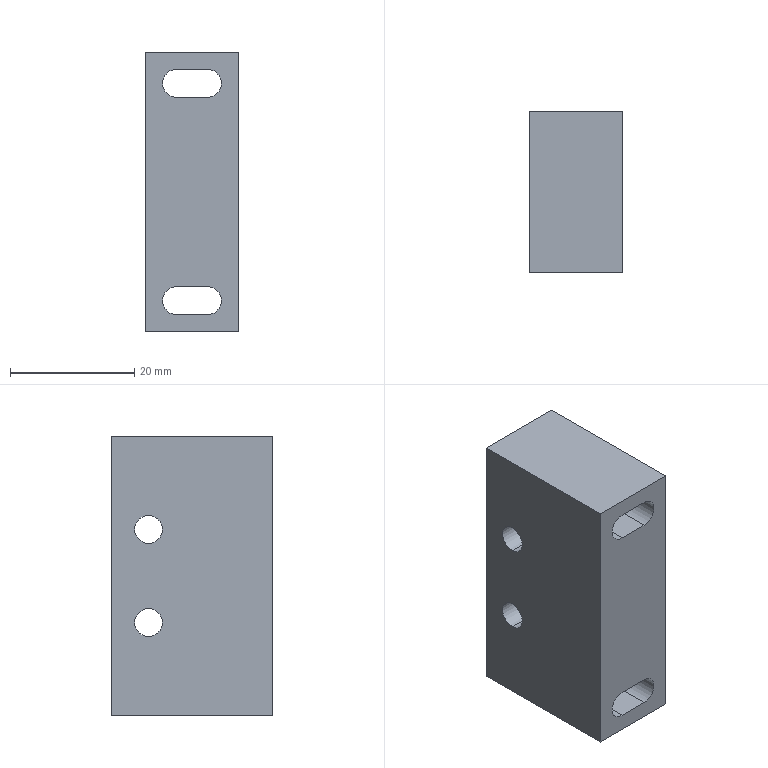Part | STEP file | 0246_221_Block | 1 solid | 18 faces | box 15 x 26 x 45 mm | volume 15076 mm3 | plane 10 | cylinder 8 | commonest cylinder face diameters 4.5 x8
STEP:
#1=CARTESIAN_POINT('',(0.,0.,0.));
#2=DIRECTION('',(0.,0.,1.));
#3=DIRECTION('',(1.,0.,0.));
#4=AXIS2_PLACEMENT_3D('',#1,#2,#3);
#5=CARTESIAN_POINT('',(-15.,20.,5.25));
#6=VERTEX_POINT('',#5);
#7=CARTESIAN_POINT('',(0.,20.,5.25));
#8=VERTEX_POINT('',#7);
#9=CARTESIAN_POINT('',(0.,20.,5.25));
#10=DIRECTION('',(1.,0.,0.));
#11=VECTOR('',#10,1.);
#12=LINE('',#9,#11);
#13=CARTESIAN_POINT('',(0.,20.,7.5));
#14=DIRECTION('',(1.,0.,0.));
#15=DIRECTION('',(0.,0.,-1.));
#16=AXIS2_PLACEMENT_3D('',#13,#14,#15);
#17=CYLINDRICAL_SURFACE('',#16,2.25);
#18=CARTESIAN_POINT('',(6.283,0.));
#19=DIRECTION('',(0.,1.));
#20=VECTOR('',#19,1.);
#21=LINE('',#18,#20);
#22=(GEOMETRIC_REPRESENTATION_CONTEXT(2)PARAMETRIC_REPRESENTATION_CONTEXT()REPRESENTATION_CONTEXT('',''));
#23=DEFINITIONAL_REPRESENTATION('',(#21),#22);
#24=PCURVE('',#17,#23);
#25=CARTESIAN_POINT('',(0.,20.,7.5));
#26=DIRECTION('',(1.,0.,0.));
#27=DIRECTION('',(0.,0.,-1.));
#28=AXIS2_PLACEMENT_3D('',#25,#26,#27);
#29=CYLINDRICAL_SURFACE('',#28,2.25);
#30=CARTESIAN_POINT('',(0.,0.));
#31=DIRECTION('',(0.,1.));
#32=VECTOR('',#31,1.);
#33=LINE('',#30,#32);
#34=(GEOMETRIC_REPRESENTATION_CONTEXT(2)PARAMETRIC_REPRESENTATION_CONTEXT()REPRESENTATION_CONTEXT('',''));
#35=DEFINITIONAL_REPRESENTATION('',(#33),#34);
#36=PCURVE('',#29,#35);
#37=SURFACE_CURVE('',#12,(#24,#36),.PCURVE_S1.);
#38=EDGE_CURVE('',#6,#8,#37,.T.);
#39=ORIENTED_EDGE('',*,*,#38,.T.);
#40=CARTESIAN_POINT('',(0.,20.,9.75));
#41=VERTEX_POINT('',#40);
#42=CARTESIAN_POINT('',(0.,20.,7.5));
#43=DIRECTION('',(1.,0.,0.));
#44=DIRECTION('',(0.,0.,-1.));
#45=AXIS2_PLACEMENT_3D('',#42,#43,#44);
#46=CIRCLE('',#45,2.25);
#47=CARTESIAN_POINT('',(0.,0.));
#48=DIRECTION('',(1.,0.));
#49=VECTOR('',#48,1.);
#50=LINE('',#47,#49);
#51=(GEOMETRIC_REPRESENTATION_CONTEXT(2)PARAMETRIC_REPRESENTATION_CONTEXT()REPRESENTATION_CONTEXT('',''));
#52=DEFINITIONAL_REPRESENTATION('',(#50),#51);
#53=PCURVE('',#17,#52);
#54=CARTESIAN_POINT('',(0.,26.,-22.5));
#55=DIRECTION('',(-1.,0.,0.));
#56=DIRECTION('',(0.,0.,1.));
#57=AXIS2_PLACEMENT_3D('',#54,#55,#56);
#58=PLANE('',#57);
#59=CARTESIAN_POINT('',(27.75,-6.));
#60=CARTESIAN_POINT('',(27.75,-2.103));
#61=CARTESIAN_POINT('',(31.125,-4.051));
#62=CARTESIAN_POINT('',(34.5,-6.));
#63=CARTESIAN_POINT('',(31.125,-7.949));
#64=CARTESIAN_POINT('',(27.75,-9.897));
#65=CARTESIAN_POINT('',(27.75,-6.));
#66=(BOUNDED_CURVE()B_SPLINE_CURVE(2,(#59,#60,#61,#62,#63,#64,#65),.UNSPECIFIED.,.T.,.F.)B_SPLINE_CURVE_WITH_KNOTS((1,2,2,2,2,1),(-2.094,0.,2.094,4.189,6.283,8.378),.UNSPECIFIED.)CURVE()GEOMETRIC_REPRESENTATION_ITEM()RATIONAL_B_SPLINE_CURVE((1.,0.5,1.,0.5,1.,0.5,1.))REPRESENTATION_ITEM(''));
#67=(GEOMETRIC_REPRESENTATION_CONTEXT(2)PARAMETRIC_REPRESENTATION_CONTEXT()REPRESENTATION_CONTEXT('',''));
#68=DEFINITIONAL_REPRESENTATION('',(#66),#67);
#69=PCURVE('',#58,#68);
#70=SURFACE_CURVE('',#46,(#53,#69),.PCURVE_S1.);
#71=EDGE_CURVE('',#41,#8,#70,.T.);
#72=ORIENTED_EDGE('',*,*,#71,.F.);
#73=CARTESIAN_POINT('',(-15.,20.,9.75));
#74=VERTEX_POINT('',#73);
#75=CARTESIAN_POINT('',(0.,20.,9.75));
#76=DIRECTION('',(1.,0.,0.));
#77=VECTOR('',#76,1.);
#78=LINE('',#75,#77);
#79=CARTESIAN_POINT('',(3.142,0.));
#80=DIRECTION('',(0.,1.));
#81=VECTOR('',#80,1.);
#82=LINE('',#79,#81);
#83=(GEOMETRIC_REPRESENTATION_CONTEXT(2)PARAMETRIC_REPRESENTATION_CONTEXT()REPRESENTATION_CONTEXT('',''));
#84=DEFINITIONAL_REPRESENTATION('',(#82),#83);
#85=PCURVE('',#17,#84);
#86=CARTESIAN_POINT('',(3.142,0.));
#87=DIRECTION('',(0.,1.));
#88=VECTOR('',#87,1.);
#89=LINE('',#86,#88);
#90=(GEOMETRIC_REPRESENTATION_CONTEXT(2)PARAMETRIC_REPRESENTATION_CONTEXT()REPRESENTATION_CONTEXT('',''));
#91=DEFINITIONAL_REPRESENTATION('',(#89),#90);
#92=PCURVE('',#29,#91);
#93=SURFACE_CURVE('',#78,(#85,#92),.PCURVE_S1.);
#94=EDGE_CURVE('',#74,#41,#93,.T.);
#95=ORIENTED_EDGE('',*,*,#94,.F.);
#96=CARTESIAN_POINT('',(-15.,20.,7.5));
#97=DIRECTION('',(1.,0.,0.));
#98=DIRECTION('',(0.,0.,-1.));
#99=AXIS2_PLACEMENT_3D('',#96,#97,#98);
#100=CIRCLE('',#99,2.25);
#101=CARTESIAN_POINT('',(0.,-15.));
#102=DIRECTION('',(1.,0.));
#103=VECTOR('',#102,1.);
#104=LINE('',#101,#103);
#105=(GEOMETRIC_REPRESENTATION_CONTEXT(2)PARAMETRIC_REPRESENTATION_CONTEXT()REPRESENTATION_CONTEXT('',''));
#106=DEFINITIONAL_REPRESENTATION('',(#104),#105);
#107=PCURVE('',#17,#106);
#108=CARTESIAN_POINT('',(-15.,26.,-22.5));
#109=DIRECTION('',(1.,0.,0.));
#110=DIRECTION('',(0.,0.,-1.));
#111=AXIS2_PLACEMENT_3D('',#108,#109,#110);
#112=PLANE('',#111);
#113=CARTESIAN_POINT('',(-30.,-6.));
#114=DIRECTION('',(1.,0.));
#115=AXIS2_PLACEMENT_2D('',#113,#114);
#116=CIRCLE('',#115,2.25);
#117=(GEOMETRIC_REPRESENTATION_CONTEXT(2)PARAMETRIC_REPRESENTATION_CONTEXT()REPRESENTATION_CONTEXT('',''));
#118=DEFINITIONAL_REPRESENTATION('',(#116),#117);
#119=PCURVE('',#112,#118);
#120=SURFACE_CURVE('',#100,(#107,#119),.PCURVE_S1.);
#121=EDGE_CURVE('',#74,#6,#120,.T.);
#122=ORIENTED_EDGE('',*,*,#121,.T.);
#123=EDGE_LOOP('',(#39,#72,#95,#122));
#124=FACE_BOUND('',#123,.F.);
#125=ADVANCED_FACE('',(#124),#17,.F.);
#126=CARTESIAN_POINT('',(-15.,20.,-9.75));
#127=VERTEX_POINT('',#126);
#128=CARTESIAN_POINT('',(0.,20.,-9.75));
#129=VERTEX_POINT('',#128);
#130=CARTESIAN_POINT('',(0.,20.,-9.75));
#131=DIRECTION('',(1.,0.,0.));
#132=VECTOR('',#131,1.);
#133=LINE('',#130,#132);
#134=CARTESIAN_POINT('',(0.,20.,-7.5));
#135=DIRECTION('',(1.,0.,0.));
#136=DIRECTION('',(0.,0.,-1.));
#137=AXIS2_PLACEMENT_3D('',#134,#135,#136);
#138=CYLINDRICAL_SURFACE('',#137,2.25);
#139=CARTESIAN_POINT('',(6.283,0.));
#140=DIRECTION('',(0.,1.));
#141=VECTOR('',#140,1.);
#142=LINE('',#139,#141);
#143=(GEOMETRIC_REPRESENTATION_CONTEXT(2)PARAMETRIC_REPRESENTATION_CONTEXT()REPRESENTATION_CONTEXT('',''));
#144=DEFINITIONAL_REPRESENTATION('',(#142),#143);
#145=PCURVE('',#138,#144);
#146=CARTESIAN_POINT('',(0.,20.,-7.5));
#147=DIRECTION('',(1.,0.,0.));
#148=DIRECTION('',(0.,0.,-1.));
#149=AXIS2_PLACEMENT_3D('',#146,#147,#148);
#150=CYLINDRICAL_SURFACE('',#149,2.25);
#151=CARTESIAN_POINT('',(0.,0.));
#152=DIRECTION('',(0.,1.));
#153=VECTOR('',#152,1.);
#154=LINE('',#151,#153);
#155=(GEOMETRIC_REPRESENTATION_CONTEXT(2)PARAMETRIC_REPRESENTATION_CONTEXT()REPRESENTATION_CONTEXT('',''));
#156=DEFINITIONAL_REPRESENTATION('',(#154),#155);
#157=PCURVE('',#150,#156);
#158=SURFACE_CURVE('',#133,(#145,#157),.PCURVE_S1.);
#159=EDGE_CURVE('',#127,#129,#158,.T.);
#160=ORIENTED_EDGE('',*,*,#159,.T.);
#161=CARTESIAN_POINT('',(0.,20.,-5.25));
#162=VERTEX_POINT('',#161);
#163=CARTESIAN_POINT('',(0.,20.,-7.5));
#164=DIRECTION('',(1.,0.,0.));
#165=DIRECTION('',(0.,0.,-1.));
#166=AXIS2_PLACEMENT_3D('',#163,#164,#165);
#167=CIRCLE('',#166,2.25);
#168=CARTESIAN_POINT('',(0.,0.));
#169=DIRECTION('',(1.,0.));
#170=VECTOR('',#169,1.);
#171=LINE('',#168,#170);
#172=(GEOMETRIC_REPRESENTATION_CONTEXT(2)PARAMETRIC_REPRESENTATION_CONTEXT()REPRESENTATION_CONTEXT('',''));
#173=DEFINITIONAL_REPRESENTATION('',(#171),#172);
#174=PCURVE('',#138,#173);
#175=CARTESIAN_POINT('',(12.75,-6.));
#176=CARTESIAN_POINT('',(12.75,-2.103));
#177=CARTESIAN_POINT('',(16.125,-4.051));
#178=CARTESIAN_POINT('',(19.5,-6.));
#179=CARTESIAN_POINT('',(16.125,-7.949));
#180=CARTESIAN_POINT('',(12.75,-9.897));
#181=CARTESIAN_POINT('',(12.75,-6.));
#182=(BOUNDED_CURVE()B_SPLINE_CURVE(2,(#175,#176,#177,#178,#179,#180,#181),.UNSPECIFIED.,.T.,.F.)B_SPLINE_CURVE_WITH_KNOTS((1,2,2,2,2,1),(-2.094,0.,2.094,4.189,6.283,8.378),.UNSPECIFIED.)CURVE()GEOMETRIC_REPRESENTATION_ITEM()RATIONAL_B_SPLINE_CURVE((1.,0.5,1.,0.5,1.,0.5,1.))REPRESENTATION_ITEM(''));
#183=(GEOMETRIC_REPRESENTATION_CONTEXT(2)PARAMETRIC_REPRESENTATION_CONTEXT()REPRESENTATION_CONTEXT('',''));
#184=DEFINITIONAL_REPRESENTATION('',(#182),#183);
#185=PCURVE('',#58,#184);
#186=SURFACE_CURVE('',#167,(#174,#185),.PCURVE_S1.);
#187=EDGE_CURVE('',#162,#129,#186,.T.);
#188=ORIENTED_EDGE('',*,*,#187,.F.);
#189=CARTESIAN_POINT('',(-15.,20.,-5.25));
#190=VERTEX_POINT('',#189);
#191=CARTESIAN_POINT('',(0.,20.,-5.25));
#192=DIRECTION('',(1.,0.,0.));
#193=VECTOR('',#192,1.);
#194=LINE('',#191,#193);
#195=CARTESIAN_POINT('',(3.142,0.));
#196=DIRECTION('',(0.,1.));
#197=VECTOR('',#196,1.);
#198=LINE('',#195,#197);
#199=(GEOMETRIC_REPRESENTATION_CONTEXT(2)PARAMETRIC_REPRESENTATION_CONTEXT()REPRESENTATION_CONTEXT('',''));
#200=DEFINITIONAL_REPRESENTATION('',(#198),#199);
#201=PCURVE('',#138,#200);
#202=CARTESIAN_POINT('',(3.142,0.));
#203=DIRECTION('',(0.,1.));
#204=VECTOR('',#203,1.);
#205=LINE('',#202,#204);
#206=(GEOMETRIC_REPRESENTATION_CONTEXT(2)PARAMETRIC_REPRESENTATION_CONTEXT()REPRESENTATION_CONTEXT('',''));
#207=DEFINITIONAL_REPRESENTATION('',(#205),#206);
#208=PCURVE('',#150,#207);
#209=SURFACE_CURVE('',#194,(#201,#208),.PCURVE_S1.);
#210=EDGE_CURVE('',#190,#162,#209,.T.);
#211=ORIENTED_EDGE('',*,*,#210,.F.);
#212=CARTESIAN_POINT('',(-15.,20.,-7.5));
#213=DIRECTION('',(1.,0.,0.));
#214=DIRECTION('',(0.,0.,-1.));
#215=AXIS2_PLACEMENT_3D('',#212,#213,#214);
#216=CIRCLE('',#215,2.25);
#217=CARTESIAN_POINT('',(0.,-15.));
#218=DIRECTION('',(1.,0.));
#219=VECTOR('',#218,1.);
#220=LINE('',#217,#219);
#221=(GEOMETRIC_REPRESENTATION_CONTEXT(2)PARAMETRIC_REPRESENTATION_CONTEXT()REPRESENTATION_CONTEXT('',''));
#222=DEFINITIONAL_REPRESENTATION('',(#220),#221);
#223=PCURVE('',#138,#222);
#224=CARTESIAN_POINT('',(-15.,-6.));
#225=DIRECTION('',(1.,0.));
#226=AXIS2_PLACEMENT_2D('',#224,#225);
#227=CIRCLE('',#226,2.25);
#228=(GEOMETRIC_REPRESENTATION_CONTEXT(2)PARAMETRIC_REPRESENTATION_CONTEXT()REPRESENTATION_CONTEXT('',''));
#229=DEFINITIONAL_REPRESENTATION('',(#227),#228);
#230=PCURVE('',#112,#229);
#231=SURFACE_CURVE('',#216,(#223,#230),.PCURVE_S1.);
#232=EDGE_CURVE('',#190,#127,#231,.T.);
#233=ORIENTED_EDGE('',*,*,#232,.T.);
#234=EDGE_LOOP('',(#160,#188,#211,#233));
#235=FACE_BOUND('',#234,.F.);
#236=ADVANCED_FACE('',(#235),#138,.F.);
#237=CARTESIAN_POINT('',(-15.,20.,7.5));
#238=DIRECTION('',(1.,0.,0.));
#239=DIRECTION('',(0.,0.,-1.));
#240=AXIS2_PLACEMENT_3D('',#237,#238,#239);
#241=CIRCLE('',#240,2.25);
#242=CARTESIAN_POINT('',(-30.,-6.));
#243=DIRECTION('',(1.,0.));
#244=AXIS2_PLACEMENT_2D('',#242,#243);
#245=CIRCLE('',#244,2.25);
#246=(GEOMETRIC_REPRESENTATION_CONTEXT(2)PARAMETRIC_REPRESENTATION_CONTEXT()REPRESENTATION_CONTEXT('',''));
#247=DEFINITIONAL_REPRESENTATION('',(#245),#246);
#248=PCURVE('',#112,#247);
#249=CARTESIAN_POINT('',(0.,-15.));
#250=DIRECTION('',(1.,0.));
#251=VECTOR('',#250,1.);
#252=LINE('',#249,#251);
#253=(GEOMETRIC_REPRESENTATION_CONTEXT(2)PARAMETRIC_REPRESENTATION_CONTEXT()REPRESENTATION_CONTEXT('',''));
#254=DEFINITIONAL_REPRESENTATION('',(#252),#253);
#255=PCURVE('',#29,#254);
#256=SURFACE_CURVE('',#241,(#248,#255),.PCURVE_S1.);
#257=EDGE_CURVE('',#6,#74,#256,.T.);
#258=ORIENTED_EDGE('',*,*,#257,.T.);
#259=ORIENTED_EDGE('',*,*,#121,.T.);
#260=EDGE_LOOP('',(#258,#259));
#261=FACE_BOUND('',#260,.T.);
#262=CARTESIAN_POINT('',(-15.,20.,-7.5));
#263=DIRECTION('',(1.,0.,0.));
#264=DIRECTION('',(0.,0.,-1.));
#265=AXIS2_PLACEMENT_3D('',#262,#263,#264);
#266=CIRCLE('',#265,2.25);
#267=CARTESIAN_POINT('',(-15.,-6.));
#268=DIRECTION('',(1.,0.));
#269=AXIS2_PLACEMENT_2D('',#267,#268);
#270=CIRCLE('',#269,2.25);
#271=(GEOMETRIC_REPRESENTATION_CONTEXT(2)PARAMETRIC_REPRESENTATION_CONTEXT()REPRESENTATION_CONTEXT('',''));
#272=DEFINITIONAL_REPRESENTATION('',(#270),#271);
#273=PCURVE('',#112,#272);
#274=CARTESIAN_POINT('',(0.,-15.));
#275=DIRECTION('',(1.,0.));
#276=VECTOR('',#275,1.);
#277=LINE('',#274,#276);
#278=(GEOMETRIC_REPRESENTATION_CONTEXT(2)PARAMETRIC_REPRESENTATION_CONTEXT()REPRESENTATION_CONTEXT('',''));
#279=DEFINITIONAL_REPRESENTATION('',(#277),#278);
#280=PCURVE('',#150,#279);
#281=SURFACE_CURVE('',#266,(#273,#280),.PCURVE_S1.);
#282=EDGE_CURVE('',#127,#190,#281,.T.);
#283=ORIENTED_EDGE('',*,*,#282,.T.);
#284=ORIENTED_EDGE('',*,*,#232,.T.);
#285=EDGE_LOOP('',(#283,#284));
#286=FACE_BOUND('',#285,.T.);
#287=CARTESIAN_POINT('',(-15.,0.,-22.5));
#288=VERTEX_POINT('',#287);
#289=CARTESIAN_POINT('',(-15.,0.,22.5));
#290=VERTEX_POINT('',#289);
#291=CARTESIAN_POINT('',(-15.,0.,-22.5));
#292=DIRECTION('',(0.,0.,1.));
#293=VECTOR('',#292,1.);
#294=LINE('',#291,#293);
#295=CARTESIAN_POINT('',(0.,-26.));
#296=DIRECTION('',(-1.,0.));
#297=VECTOR('',#296,1.);
#298=LINE('',#295,#297);
#299=(GEOMETRIC_REPRESENTATION_CONTEXT(2)PARAMETRIC_REPRESENTATION_CONTEXT()REPRESENTATION_CONTEXT('',''));
#300=DEFINITIONAL_REPRESENTATION('',(#298),#299);
#301=PCURVE('',#112,#300);
#302=CARTESIAN_POINT('',(-15.,0.,22.5));
#303=DIRECTION('',(0.,1.,0.));
#304=DIRECTION('',(0.,0.,1.));
#305=AXIS2_PLACEMENT_3D('',#302,#303,#304);
#306=PLANE('',#305);
#307=CARTESIAN_POINT('',(-45.,0.));
#308=DIRECTION('',(1.,0.));
#309=VECTOR('',#308,1.);
#310=LINE('',#307,#309);
#311=(GEOMETRIC_REPRESENTATION_CONTEXT(2)PARAMETRIC_REPRESENTATION_CONTEXT()REPRESENTATION_CONTEXT('',''));
#312=DEFINITIONAL_REPRESENTATION('',(#310),#311);
#313=PCURVE('',#306,#312);
#314=SURFACE_CURVE('',#294,(#301,#313),.PCURVE_S1.);
#315=EDGE_CURVE('',#288,#290,#314,.T.);
#316=ORIENTED_EDGE('',*,*,#315,.T.);
#317=CARTESIAN_POINT('',(-15.,26.,22.5));
#318=VERTEX_POINT('',#317);
#319=CARTESIAN_POINT('',(-15.,26.,22.5));
#320=DIRECTION('',(0.,-1.,0.));
#321=VECTOR('',#320,1.);
#322=LINE('',#319,#321);
#323=CARTESIAN_POINT('',(-45.,0.));
#324=DIRECTION('',(0.,-1.));
#325=VECTOR('',#324,1.);
#326=LINE('',#323,#325);
#327=(GEOMETRIC_REPRESENTATION_CONTEXT(2)PARAMETRIC_REPRESENTATION_CONTEXT()REPRESENTATION_CONTEXT('',''));
#328=DEFINITIONAL_REPRESENTATION('',(#326),#327);
#329=PCURVE('',#112,#328);
#330=CARTESIAN_POINT('',(-15.,26.,22.5));
#331=DIRECTION('',(0.,0.,-1.));
#332=DIRECTION('',(-1.,0.,0.));
#333=AXIS2_PLACEMENT_3D('',#330,#331,#332);
#334=PLANE('',#333);
#335=CARTESIAN_POINT('',(0.,0.));
#336=DIRECTION('',(0.,-1.));
#337=VECTOR('',#336,1.);
#338=LINE('',#335,#337);
#339=(GEOMETRIC_REPRESENTATION_CONTEXT(2)PARAMETRIC_REPRESENTATION_CONTEXT()REPRESENTATION_CONTEXT('',''));
#340=DEFINITIONAL_REPRESENTATION('',(#338),#339);
#341=PCURVE('',#334,#340);
#342=SURFACE_CURVE('',#322,(#329,#341),.PCURVE_S1.);
#343=EDGE_CURVE('',#318,#290,#342,.T.);
#344=ORIENTED_EDGE('',*,*,#343,.F.);
#345=CARTESIAN_POINT('',(-15.,26.,-22.5));
#346=VERTEX_POINT('',#345);
#347=CARTESIAN_POINT('',(-15.,26.,-22.5));
#348=DIRECTION('',(0.,0.,1.));
#349=VECTOR('',#348,1.);
#350=LINE('',#347,#349);
#351=CARTESIAN_POINT('',(0.,0.));
#352=DIRECTION('',(-1.,0.));
#353=VECTOR('',#352,1.);
#354=LINE('',#351,#353);
#355=(GEOMETRIC_REPRESENTATION_CONTEXT(2)PARAMETRIC_REPRESENTATION_CONTEXT()REPRESENTATION_CONTEXT('',''));
#356=DEFINITIONAL_REPRESENTATION('',(#354),#355);
#357=PCURVE('',#112,#356);
#358=CARTESIAN_POINT('',(-15.,26.,22.5));
#359=DIRECTION('',(0.,1.,0.));
#360=DIRECTION('',(0.,0.,1.));
#361=AXIS2_PLACEMENT_3D('',#358,#359,#360);
#362=PLANE('',#361);
#363=CARTESIAN_POINT('',(-45.,0.));
#364=DIRECTION('',(1.,0.));
#365=VECTOR('',#364,1.);
#366=LINE('',#363,#365);
#367=(GEOMETRIC_REPRESENTATION_CONTEXT(2)PARAMETRIC_REPRESENTATION_CONTEXT()REPRESENTATION_CONTEXT('',''));
#368=DEFINITIONAL_REPRESENTATION('',(#366),#367);
#369=PCURVE('',#362,#368);
#370=SURFACE_CURVE('',#350,(#357,#369),.PCURVE_S1.);
#371=EDGE_CURVE('',#346,#318,#370,.T.);
#372=ORIENTED_EDGE('',*,*,#371,.F.);
#373=CARTESIAN_POINT('',(-15.,26.,-22.5));
#374=DIRECTION('',(0.,-1.,0.));
#375=VECTOR('',#374,1.);
#376=LINE('',#373,#375);
#377=CARTESIAN_POINT('',(0.,0.));
#378=DIRECTION('',(0.,-1.));
#379=VECTOR('',#378,1.);
#380=LINE('',#377,#379);
#381=(GEOMETRIC_REPRESENTATION_CONTEXT(2)PARAMETRIC_REPRESENTATION_CONTEXT()REPRESENTATION_CONTEXT('',''));
#382=DEFINITIONAL_REPRESENTATION('',(#380),#381);
#383=PCURVE('',#112,#382);
#384=CARTESIAN_POINT('',(-15.,26.,-22.5));
#385=DIRECTION('',(0.,0.,1.));
#386=DIRECTION('',(1.,0.,0.));
#387=AXIS2_PLACEMENT_3D('',#384,#385,#386);
#388=PLANE('',#387);
#389=CARTESIAN_POINT('',(0.,0.));
#390=DIRECTION('',(0.,-1.));
#391=VECTOR('',#390,1.);
#392=LINE('',#389,#391);
#393=(GEOMETRIC_REPRESENTATION_CONTEXT(2)PARAMETRIC_REPRESENTATION_CONTEXT()REPRESENTATION_CONTEXT('',''));
#394=DEFINITIONAL_REPRESENTATION('',(#392),#393);
#395=PCURVE('',#388,#394);
#396=SURFACE_CURVE('',#376,(#383,#395),.PCURVE_S1.);
#397=EDGE_CURVE('',#346,#288,#396,.T.);
#398=ORIENTED_EDGE('',*,*,#397,.T.);
#399=EDGE_LOOP('',(#316,#344,#372,#398));
#400=FACE_BOUND('',#399,.T.);
#401=ADVANCED_FACE('',(#261,#286,#400),#112,.F.);
#402=CARTESIAN_POINT('',(0.,0.,22.5));
#403=VERTEX_POINT('',#402);
#404=CARTESIAN_POINT('',(-15.,0.,22.5));
#405=DIRECTION('',(1.,0.,0.));
#406=VECTOR('',#405,1.);
#407=LINE('',#404,#406);
#408=CARTESIAN_POINT('',(0.,-26.));
#409=DIRECTION('',(-1.,0.));
#410=VECTOR('',#409,1.);
#411=LINE('',#408,#410);
#412=(GEOMETRIC_REPRESENTATION_CONTEXT(2)PARAMETRIC_REPRESENTATION_CONTEXT()REPRESENTATION_CONTEXT('',''));
#413=DEFINITIONAL_REPRESENTATION('',(#411),#412);
#414=PCURVE('',#334,#413);
#415=CARTESIAN_POINT('',(0.,0.));
#416=DIRECTION('',(0.,1.));
#417=VECTOR('',#416,1.);
#418=LINE('',#415,#417);
#419=(GEOMETRIC_REPRESENTATION_CONTEXT(2)PARAMETRIC_REPRESENTATION_CONTEXT()REPRESENTATION_CONTEXT('',''));
#420=DEFINITIONAL_REPRESENTATION('',(#418),#419);
#421=PCURVE('',#306,#420);
#422=SURFACE_CURVE('',#407,(#414,#421),.PCURVE_S1.);
#423=EDGE_CURVE('',#290,#403,#422,.T.);
#424=ORIENTED_EDGE('',*,*,#423,.T.);
#425=CARTESIAN_POINT('',(0.,26.,22.5));
#426=VERTEX_POINT('',#425);
#427=CARTESIAN_POINT('',(0.,26.,22.5));
#428=DIRECTION('',(0.,-1.,0.));
#429=VECTOR('',#428,1.);
#430=LINE('',#427,#429);
#431=CARTESIAN_POINT('',(-15.,0.));
#432=DIRECTION('',(0.,-1.));
#433=VECTOR('',#432,1.);
#434=LINE('',#431,#433);
#435=(GEOMETRIC_REPRESENTATION_CONTEXT(2)PARAMETRIC_REPRESENTATION_CONTEXT()REPRESENTATION_CONTEXT('',''));
#436=DEFINITIONAL_REPRESENTATION('',(#434),#435);
#437=PCURVE('',#334,#436);
#438=CARTESIAN_POINT('',(45.,0.));
#439=DIRECTION('',(0.,-1.));
#440=VECTOR('',#439,1.);
#441=LINE('',#438,#440);
#442=(GEOMETRIC_REPRESENTATION_CONTEXT(2)PARAMETRIC_REPRESENTATION_CONTEXT()REPRESENTATION_CONTEXT('',''));
#443=DEFINITIONAL_REPRESENTATION('',(#441),#442);
#444=PCURVE('',#58,#443);
#445=SURFACE_CURVE('',#430,(#437,#444),.PCURVE_S1.);
#446=EDGE_CURVE('',#426,#403,#445,.T.);
#447=ORIENTED_EDGE('',*,*,#446,.F.);
#448=CARTESIAN_POINT('',(-15.,26.,22.5));
#449=DIRECTION('',(1.,0.,0.));
#450=VECTOR('',#449,1.);
#451=LINE('',#448,#450);
#452=CARTESIAN_POINT('',(0.,0.));
#453=DIRECTION('',(-1.,0.));
#454=VECTOR('',#453,1.);
#455=LINE('',#452,#454);
#456=(GEOMETRIC_REPRESENTATION_CONTEXT(2)PARAMETRIC_REPRESENTATION_CONTEXT()REPRESENTATION_CONTEXT('',''));
#457=DEFINITIONAL_REPRESENTATION('',(#455),#456);
#458=PCURVE('',#334,#457);
#459=CARTESIAN_POINT('',(0.,0.));
#460=DIRECTION('',(0.,1.));
#461=VECTOR('',#460,1.);
#462=LINE('',#459,#461);
#463=(GEOMETRIC_REPRESENTATION_CONTEXT(2)PARAMETRIC_REPRESENTATION_CONTEXT()REPRESENTATION_CONTEXT('',''));
#464=DEFINITIONAL_REPRESENTATION('',(#462),#463);
#465=PCURVE('',#362,#464);
#466=SURFACE_CURVE('',#451,(#458,#465),.PCURVE_S1.);
#467=EDGE_CURVE('',#318,#426,#466,.T.);
#468=ORIENTED_EDGE('',*,*,#467,.F.);
#469=ORIENTED_EDGE('',*,*,#343,.T.);
#470=EDGE_LOOP('',(#424,#447,#468,#469));
#471=FACE_BOUND('',#470,.T.);
#472=ADVANCED_FACE('',(#471),#334,.F.);
#473=CARTESIAN_POINT('',(0.,20.,7.5));
#474=DIRECTION('',(1.,0.,0.));
#475=DIRECTION('',(0.,0.,-1.));
#476=AXIS2_PLACEMENT_3D('',#473,#474,#475);
#477=CIRCLE('',#476,2.25);
#478=CARTESIAN_POINT('',(27.75,-6.));
#479=CARTESIAN_POINT('',(27.75,-2.103));
#480=CARTESIAN_POINT('',(31.125,-4.051));
#481=CARTESIAN_POINT('',(34.5,-6.));
#482=CARTESIAN_POINT('',(31.125,-7.949));
#483=CARTESIAN_POINT('',(27.75,-9.897));
#484=CARTESIAN_POINT('',(27.75,-6.));
#485=(BOUNDED_CURVE()B_SPLINE_CURVE(2,(#478,#479,#480,#481,#482,#483,#484),.UNSPECIFIED.,.T.,.F.)B_SPLINE_CURVE_WITH_KNOTS((1,2,2,2,2,1),(-2.094,0.,2.094,4.189,6.283,8.378),.UNSPECIFIED.)CURVE()GEOMETRIC_REPRESENTATION_ITEM()RATIONAL_B_SPLINE_CURVE((1.,0.5,1.,0.5,1.,0.5,1.))REPRESENTATION_ITEM(''));
#486=(GEOMETRIC_REPRESENTATION_CONTEXT(2)PARAMETRIC_REPRESENTATION_CONTEXT()REPRESENTATION_CONTEXT('',''));
#487=DEFINITIONAL_REPRESENTATION('',(#485),#486);
#488=PCURVE('',#58,#487);
#489=CARTESIAN_POINT('',(0.,0.));
#490=DIRECTION('',(1.,0.));
#491=VECTOR('',#490,1.);
#492=LINE('',#489,#491);
#493=(GEOMETRIC_REPRESENTATION_CONTEXT(2)PARAMETRIC_REPRESENTATION_CONTEXT()REPRESENTATION_CONTEXT('',''));
#494=DEFINITIONAL_REPRESENTATION('',(#492),#493);
#495=PCURVE('',#29,#494);
#496=SURFACE_CURVE('',#477,(#488,#495),.PCURVE_S1.);
#497=EDGE_CURVE('',#8,#41,#496,.T.);
#498=ORIENTED_EDGE('',*,*,#497,.F.);
#499=ORIENTED_EDGE('',*,*,#71,.F.);
#500=EDGE_LOOP('',(#498,#499));
#501=FACE_BOUND('',#500,.T.);
#502=CARTESIAN_POINT('',(0.,20.,-7.5));
#503=DIRECTION('',(1.,0.,0.));
#504=DIRECTION('',(0.,0.,-1.));
#505=AXIS2_PLACEMENT_3D('',#502,#503,#504);
#506=CIRCLE('',#505,2.25);
#507=CARTESIAN_POINT('',(12.75,-6.));
#508=CARTESIAN_POINT('',(12.75,-2.103));
#509=CARTESIAN_POINT('',(16.125,-4.051));
#510=CARTESIAN_POINT('',(19.5,-6.));
#511=CARTESIAN_POINT('',(16.125,-7.949));
#512=CARTESIAN_POINT('',(12.75,-9.897));
#513=CARTESIAN_POINT('',(12.75,-6.));
#514=(BOUNDED_CURVE()B_SPLINE_CURVE(2,(#507,#508,#509,#510,#511,#512,#513),.UNSPECIFIED.,.T.,.F.)B_SPLINE_CURVE_WITH_KNOTS((1,2,2,2,2,1),(-2.094,0.,2.094,4.189,6.283,8.378),.UNSPECIFIED.)CURVE()GEOMETRIC_REPRESENTATION_ITEM()RATIONAL_B_SPLINE_CURVE((1.,0.5,1.,0.5,1.,0.5,1.))REPRESENTATION_ITEM(''));
#515=(GEOMETRIC_REPRESENTATION_CONTEXT(2)PARAMETRIC_REPRESENTATION_CONTEXT()REPRESENTATION_CONTEXT('',''));
#516=DEFINITIONAL_REPRESENTATION('',(#514),#515);
#517=PCURVE('',#58,#516);
#518=CARTESIAN_POINT('',(0.,0.));
#519=DIRECTION('',(1.,0.));
#520=VECTOR('',#519,1.);
#521=LINE('',#518,#520);
#522=(GEOMETRIC_REPRESENTATION_CONTEXT(2)PARAMETRIC_REPRESENTATION_CONTEXT()REPRESENTATION_CONTEXT('',''));
#523=DEFINITIONAL_REPRESENTATION('',(#521),#522);
#524=PCURVE('',#150,#523);
#525=SURFACE_CURVE('',#506,(#517,#524),.PCURVE_S1.);
#526=EDGE_CURVE('',#129,#162,#525,.T.);
#527=ORIENTED_EDGE('',*,*,#526,.F.);
#528=ORIENTED_EDGE('',*,*,#187,.F.);
#529=EDGE_LOOP('',(#527,#528));
#530=FACE_BOUND('',#529,.T.);
#531=CARTESIAN_POINT('',(0.,0.,-22.5));
#532=VERTEX_POINT('',#531);
#533=CARTESIAN_POINT('',(0.,0.,-22.5));
#534=DIRECTION('',(0.,0.,-1.));
#535=VECTOR('',#534,1.);
#536=LINE('',#533,#535);
#537=CARTESIAN_POINT('',(0.,-26.));
#538=DIRECTION('',(-1.,0.));
#539=VECTOR('',#538,1.);
#540=LINE('',#537,#539);
#541=(GEOMETRIC_REPRESENTATION_CONTEXT(2)PARAMETRIC_REPRESENTATION_CONTEXT()REPRESENTATION_CONTEXT('',''));
#542=DEFINITIONAL_REPRESENTATION('',(#540),#541);
#543=PCURVE('',#58,#542);
#544=CARTESIAN_POINT('',(-45.,15.));
#545=DIRECTION('',(-1.,0.));
#546=VECTOR('',#545,1.);
#547=LINE('',#544,#546);
#548=(GEOMETRIC_REPRESENTATION_CONTEXT(2)PARAMETRIC_REPRESENTATION_CONTEXT()REPRESENTATION_CONTEXT('',''));
#549=DEFINITIONAL_REPRESENTATION('',(#547),#548);
#550=PCURVE('',#306,#549);
#551=SURFACE_CURVE('',#536,(#543,#550),.PCURVE_S1.);
#552=EDGE_CURVE('',#403,#532,#551,.T.);
#553=ORIENTED_EDGE('',*,*,#552,.T.);
#554=CARTESIAN_POINT('',(0.,26.,-22.5));
#555=VERTEX_POINT('',#554);
#556=CARTESIAN_POINT('',(0.,26.,-22.5));
#557=DIRECTION('',(0.,-1.,0.));
#558=VECTOR('',#557,1.);
#559=LINE('',#556,#558);
#560=CARTESIAN_POINT('',(0.,0.));
#561=DIRECTION('',(0.,-1.));
#562=VECTOR('',#561,1.);
#563=LINE('',#560,#562);
#564=(GEOMETRIC_REPRESENTATION_CONTEXT(2)PARAMETRIC_REPRESENTATION_CONTEXT()REPRESENTATION_CONTEXT('',''));
#565=DEFINITIONAL_REPRESENTATION('',(#563),#564);
#566=PCURVE('',#58,#565);
#567=CARTESIAN_POINT('',(15.,0.));
#568=DIRECTION('',(0.,-1.));
#569=VECTOR('',#568,1.);
#570=LINE('',#567,#569);
#571=(GEOMETRIC_REPRESENTATION_CONTEXT(2)PARAMETRIC_REPRESENTATION_CONTEXT()REPRESENTATION_CONTEXT('',''));
#572=DEFINITIONAL_REPRESENTATION('',(#570),#571);
#573=PCURVE('',#388,#572);
#574=SURFACE_CURVE('',#559,(#566,#573),.PCURVE_S1.);
#575=EDGE_CURVE('',#555,#532,#574,.T.);
#576=ORIENTED_EDGE('',*,*,#575,.F.);
#577=CARTESIAN_POINT('',(0.,26.,-22.5));
#578=DIRECTION('',(0.,0.,-1.));
#579=VECTOR('',#578,1.);
#580=LINE('',#577,#579);
#581=CARTESIAN_POINT('',(0.,0.));
#582=DIRECTION('',(-1.,0.));
#583=VECTOR('',#582,1.);
#584=LINE('',#581,#583);
#585=(GEOMETRIC_REPRESENTATION_CONTEXT(2)PARAMETRIC_REPRESENTATION_CONTEXT()REPRESENTATION_CONTEXT('',''));
#586=DEFINITIONAL_REPRESENTATION('',(#584),#585);
#587=PCURVE('',#58,#586);
#588=CARTESIAN_POINT('',(-45.,15.));
#589=DIRECTION('',(-1.,0.));
#590=VECTOR('',#589,1.);
#591=LINE('',#588,#590);
#592=(GEOMETRIC_REPRESENTATION_CONTEXT(2)PARAMETRIC_REPRESENTATION_CONTEXT()REPRESENTATION_CONTEXT('',''));
#593=DEFINITIONAL_REPRESENTATION('',(#591),#592);
#594=PCURVE('',#362,#593);
#595=SURFACE_CURVE('',#580,(#587,#594),.PCURVE_S1.);
#596=EDGE_CURVE('',#426,#555,#595,.T.);
#597=ORIENTED_EDGE('',*,*,#596,.F.);
#598=ORIENTED_EDGE('',*,*,#446,.T.);
#599=EDGE_LOOP('',(#553,#576,#597,#598));
#600=FACE_BOUND('',#599,.T.);
#601=ADVANCED_FACE('',(#501,#530,#600),#58,.F.);
#602=CARTESIAN_POINT('',(-15.,0.,-22.5));
#603=DIRECTION('',(-1.,0.,0.));
#604=VECTOR('',#603,1.);
#605=LINE('',#602,#604);
#606=CARTESIAN_POINT('',(0.,-26.));
#607=DIRECTION('',(-1.,0.));
#608=VECTOR('',#607,1.);
#609=LINE('',#606,#608);
#610=(GEOMETRIC_REPRESENTATION_CONTEXT(2)PARAMETRIC_REPRESENTATION_CONTEXT()REPRESENTATION_CONTEXT('',''));
#611=DEFINITIONAL_REPRESENTATION('',(#609),#610);
#612=PCURVE('',#388,#611);
#613=CARTESIAN_POINT('',(-45.,0.));
#614=DIRECTION('',(0.,-1.));
#615=VECTOR('',#614,1.);
#616=LINE('',#613,#615);
#617=(GEOMETRIC_REPRESENTATION_CONTEXT(2)PARAMETRIC_REPRESENTATION_CONTEXT()REPRESENTATION_CONTEXT('',''));
#618=DEFINITIONAL_REPRESENTATION('',(#616),#617);
#619=PCURVE('',#306,#618);
#620=SURFACE_CURVE('',#605,(#612,#619),.PCURVE_S1.);
#621=EDGE_CURVE('',#532,#288,#620,.T.);
#622=ORIENTED_EDGE('',*,*,#621,.T.);
#623=ORIENTED_EDGE('',*,*,#397,.F.);
#624=CARTESIAN_POINT('',(-15.,26.,-22.5));
#625=DIRECTION('',(-1.,0.,0.));
#626=VECTOR('',#625,1.);
#627=LINE('',#624,#626);
#628=CARTESIAN_POINT('',(0.,0.));
#629=DIRECTION('',(-1.,0.));
#630=VECTOR('',#629,1.);
#631=LINE('',#628,#630);
#632=(GEOMETRIC_REPRESENTATION_CONTEXT(2)PARAMETRIC_REPRESENTATION_CONTEXT()REPRESENTATION_CONTEXT('',''));
#633=DEFINITIONAL_REPRESENTATION('',(#631),#632);
#634=PCURVE('',#388,#633);
#635=CARTESIAN_POINT('',(-45.,0.));
#636=DIRECTION('',(0.,-1.));
#637=VECTOR('',#636,1.);
#638=LINE('',#635,#637);
#639=(GEOMETRIC_REPRESENTATION_CONTEXT(2)PARAMETRIC_REPRESENTATION_CONTEXT()REPRESENTATION_CONTEXT('',''));
#640=DEFINITIONAL_REPRESENTATION('',(#638),#639);
#641=PCURVE('',#362,#640);
#642=SURFACE_CURVE('',#627,(#634,#641),.PCURVE_S1.);
#643=EDGE_CURVE('',#555,#346,#642,.T.);
#644=ORIENTED_EDGE('',*,*,#643,.F.);
#645=ORIENTED_EDGE('',*,*,#575,.T.);
#646=EDGE_LOOP('',(#622,#623,#644,#645));
#647=FACE_BOUND('',#646,.T.);
#648=ADVANCED_FACE('',(#647),#388,.F.);
#649=CARTESIAN_POINT('',(-10.,26.,15.25));
#650=VERTEX_POINT('',#649);
#651=CARTESIAN_POINT('',(-10.,26.,19.75));
#652=VERTEX_POINT('',#651);
#653=CARTESIAN_POINT('',(-10.,26.,17.5));
#654=DIRECTION('',(0.,1.,0.));
#655=DIRECTION('',(0.,0.,1.));
#656=AXIS2_PLACEMENT_3D('',#653,#654,#655);
#657=CIRCLE('',#656,2.25);
#658=CARTESIAN_POINT('',(-5.,5.));
#659=DIRECTION('',(1.,0.));
#660=AXIS2_PLACEMENT_2D('',#658,#659);
#661=CIRCLE('',#660,2.25);
#662=(GEOMETRIC_REPRESENTATION_CONTEXT(2)PARAMETRIC_REPRESENTATION_CONTEXT()REPRESENTATION_CONTEXT('',''));
#663=DEFINITIONAL_REPRESENTATION('',(#661),#662);
#664=PCURVE('',#362,#663);
#665=CARTESIAN_POINT('',(-10.,0.,17.5));
#666=DIRECTION('',(0.,1.,0.));
#667=DIRECTION('',(0.,0.,1.));
#668=AXIS2_PLACEMENT_3D('',#665,#666,#667);
#669=CYLINDRICAL_SURFACE('',#668,2.25);
#670=CARTESIAN_POINT('',(0.,26.));
#671=DIRECTION('',(1.,0.));
#672=VECTOR('',#671,1.);
#673=LINE('',#670,#672);
#674=(GEOMETRIC_REPRESENTATION_CONTEXT(2)PARAMETRIC_REPRESENTATION_CONTEXT()REPRESENTATION_CONTEXT('',''));
#675=DEFINITIONAL_REPRESENTATION('',(#673),#674);
#676=PCURVE('',#669,#675);
#677=SURFACE_CURVE('',#657,(#664,#676),.PCURVE_S1.);
#678=EDGE_CURVE('',#650,#652,#677,.T.);
#679=ORIENTED_EDGE('',*,*,#678,.F.);
#680=CARTESIAN_POINT('',(-5.,26.,15.25));
#681=VERTEX_POINT('',#680);
#682=CARTESIAN_POINT('',(-10.,26.,15.25));
#683=DIRECTION('',(-1.,0.,0.));
#684=VECTOR('',#683,1.);
#685=LINE('',#682,#684);
#686=CARTESIAN_POINT('',(-7.25,5.));
#687=DIRECTION('',(0.,-1.));
#688=VECTOR('',#687,1.);
#689=LINE('',#686,#688);
#690=(GEOMETRIC_REPRESENTATION_CONTEXT(2)PARAMETRIC_REPRESENTATION_CONTEXT()REPRESENTATION_CONTEXT('',''));
#691=DEFINITIONAL_REPRESENTATION('',(#689),#690);
#692=PCURVE('',#362,#691);
#693=CARTESIAN_POINT('',(-10.,0.,15.25));
#694=DIRECTION('',(0.,0.,-1.));
#695=DIRECTION('',(-1.,0.,0.));
#696=AXIS2_PLACEMENT_3D('',#693,#694,#695);
#697=PLANE('',#696);
#698=CARTESIAN_POINT('',(0.,26.));
#699=DIRECTION('',(1.,0.));
#700=VECTOR('',#699,1.);
#701=LINE('',#698,#700);
#702=(GEOMETRIC_REPRESENTATION_CONTEXT(2)PARAMETRIC_REPRESENTATION_CONTEXT()REPRESENTATION_CONTEXT('',''));
#703=DEFINITIONAL_REPRESENTATION('',(#701),#702);
#704=PCURVE('',#697,#703);
#705=SURFACE_CURVE('',#685,(#692,#704),.PCURVE_S1.);
#706=EDGE_CURVE('',#681,#650,#705,.T.);
#707=ORIENTED_EDGE('',*,*,#706,.F.);
#708=CARTESIAN_POINT('',(-5.,26.,19.75));
#709=VERTEX_POINT('',#708);
#710=CARTESIAN_POINT('',(-5.,26.,17.5));
#711=DIRECTION('',(0.,1.,0.));
#712=DIRECTION('',(0.,0.,1.));
#713=AXIS2_PLACEMENT_3D('',#710,#711,#712);
#714=CIRCLE('',#713,2.25);
#715=CARTESIAN_POINT('',(-5.,10.));
#716=DIRECTION('',(1.,0.));
#717=AXIS2_PLACEMENT_2D('',#715,#716);
#718=CIRCLE('',#717,2.25);
#719=(GEOMETRIC_REPRESENTATION_CONTEXT(2)PARAMETRIC_REPRESENTATION_CONTEXT()REPRESENTATION_CONTEXT('',''));
#720=DEFINITIONAL_REPRESENTATION('',(#718),#719);
#721=PCURVE('',#362,#720);
#722=CARTESIAN_POINT('',(-5.,0.,17.5));
#723=DIRECTION('',(0.,1.,0.));
#724=DIRECTION('',(0.,0.,1.));
#725=AXIS2_PLACEMENT_3D('',#722,#723,#724);
#726=CYLINDRICAL_SURFACE('',#725,2.25);
#727=CARTESIAN_POINT('',(0.,26.));
#728=DIRECTION('',(1.,0.));
#729=VECTOR('',#728,1.);
#730=LINE('',#727,#729);
#731=(GEOMETRIC_REPRESENTATION_CONTEXT(2)PARAMETRIC_REPRESENTATION_CONTEXT()REPRESENTATION_CONTEXT('',''));
#732=DEFINITIONAL_REPRESENTATION('',(#730),#731);
#733=PCURVE('',#726,#732);
#734=SURFACE_CURVE('',#714,(#721,#733),.PCURVE_S1.);
#735=EDGE_CURVE('',#709,#681,#734,.T.);
#736=ORIENTED_EDGE('',*,*,#735,.F.);
#737=CARTESIAN_POINT('',(-10.,26.,19.75));
#738=DIRECTION('',(1.,0.,0.));
#739=VECTOR('',#738,1.);
#740=LINE('',#737,#739);
#741=CARTESIAN_POINT('',(-2.75,5.));
#742=DIRECTION('',(0.,1.));
#743=VECTOR('',#742,1.);
#744=LINE('',#741,#743);
#745=(GEOMETRIC_REPRESENTATION_CONTEXT(2)PARAMETRIC_REPRESENTATION_CONTEXT()REPRESENTATION_CONTEXT('',''));
#746=DEFINITIONAL_REPRESENTATION('',(#744),#745);
#747=PCURVE('',#362,#746);
#748=CARTESIAN_POINT('',(-10.,0.,19.75));
#749=DIRECTION('',(0.,0.,1.));
#750=DIRECTION('',(1.,0.,0.));
#751=AXIS2_PLACEMENT_3D('',#748,#749,#750);
#752=PLANE('',#751);
#753=CARTESIAN_POINT('',(0.,26.));
#754=DIRECTION('',(1.,0.));
#755=VECTOR('',#754,1.);
#756=LINE('',#753,#755);
#757=(GEOMETRIC_REPRESENTATION_CONTEXT(2)PARAMETRIC_REPRESENTATION_CONTEXT()REPRESENTATION_CONTEXT('',''));
#758=DEFINITIONAL_REPRESENTATION('',(#756),#757);
#759=PCURVE('',#752,#758);
#760=SURFACE_CURVE('',#740,(#747,#759),.PCURVE_S1.);
#761=EDGE_CURVE('',#652,#709,#760,.T.);
#762=ORIENTED_EDGE('',*,*,#761,.F.);
#763=EDGE_LOOP('',(#679,#707,#736,#762));
#764=FACE_BOUND('',#763,.T.);
#765=CARTESIAN_POINT('',(-10.,26.,-19.75));
#766=VERTEX_POINT('',#765);
#767=CARTESIAN_POINT('',(-10.,26.,-15.25));
#768=VERTEX_POINT('',#767);
#769=CARTESIAN_POINT('',(-10.,26.,-17.5));
#770=DIRECTION('',(0.,1.,0.));
#771=DIRECTION('',(0.,0.,1.));
#772=AXIS2_PLACEMENT_3D('',#769,#770,#771);
#773=CIRCLE('',#772,2.25);
#774=CARTESIAN_POINT('',(-40.,5.));
#775=DIRECTION('',(1.,0.));
#776=AXIS2_PLACEMENT_2D('',#774,#775);
#777=CIRCLE('',#776,2.25);
#778=(GEOMETRIC_REPRESENTATION_CONTEXT(2)PARAMETRIC_REPRESENTATION_CONTEXT()REPRESENTATION_CONTEXT('',''));
#779=DEFINITIONAL_REPRESENTATION('',(#777),#778);
#780=PCURVE('',#362,#779);
#781=CARTESIAN_POINT('',(-10.,0.,-17.5));
#782=DIRECTION('',(0.,1.,0.));
#783=DIRECTION('',(0.,0.,1.));
#784=AXIS2_PLACEMENT_3D('',#781,#782,#783);
#785=CYLINDRICAL_SURFACE('',#784,2.25);
#786=CARTESIAN_POINT('',(0.,26.));
#787=DIRECTION('',(1.,0.));
#788=VECTOR('',#787,1.);
#789=LINE('',#786,#788);
#790=(GEOMETRIC_REPRESENTATION_CONTEXT(2)PARAMETRIC_REPRESENTATION_CONTEXT()REPRESENTATION_CONTEXT('',''));
#791=DEFINITIONAL_REPRESENTATION('',(#789),#790);
#792=PCURVE('',#785,#791);
#793=SURFACE_CURVE('',#773,(#780,#792),.PCURVE_S1.);
#794=EDGE_CURVE('',#766,#768,#793,.T.);
#795=ORIENTED_EDGE('',*,*,#794,.F.);
#796=CARTESIAN_POINT('',(-5.,26.,-19.75));
#797=VERTEX_POINT('',#796);
#798=CARTESIAN_POINT('',(-10.,26.,-19.75));
#799=DIRECTION('',(-1.,0.,0.));
#800=VECTOR('',#799,1.);
#801=LINE('',#798,#800);
#802=CARTESIAN_POINT('',(-42.25,5.));
#803=DIRECTION('',(0.,-1.));
#804=VECTOR('',#803,1.);
#805=LINE('',#802,#804);
#806=(GEOMETRIC_REPRESENTATION_CONTEXT(2)PARAMETRIC_REPRESENTATION_CONTEXT()REPRESENTATION_CONTEXT('',''));
#807=DEFINITIONAL_REPRESENTATION('',(#805),#806);
#808=PCURVE('',#362,#807);
#809=CARTESIAN_POINT('',(-10.,0.,-19.75));
#810=DIRECTION('',(0.,0.,-1.));
#811=DIRECTION('',(-1.,0.,0.));
#812=AXIS2_PLACEMENT_3D('',#809,#810,#811);
#813=PLANE('',#812);
#814=CARTESIAN_POINT('',(0.,26.));
#815=DIRECTION('',(1.,0.));
#816=VECTOR('',#815,1.);
#817=LINE('',#814,#816);
#818=(GEOMETRIC_REPRESENTATION_CONTEXT(2)PARAMETRIC_REPRESENTATION_CONTEXT()REPRESENTATION_CONTEXT('',''));
#819=DEFINITIONAL_REPRESENTATION('',(#817),#818);
#820=PCURVE('',#813,#819);
#821=SURFACE_CURVE('',#801,(#808,#820),.PCURVE_S1.);
#822=EDGE_CURVE('',#797,#766,#821,.T.);
#823=ORIENTED_EDGE('',*,*,#822,.F.);
#824=CARTESIAN_POINT('',(-5.,26.,-15.25));
#825=VERTEX_POINT('',#824);
#826=CARTESIAN_POINT('',(-5.,26.,-17.5));
#827=DIRECTION('',(0.,1.,0.));
#828=DIRECTION('',(0.,0.,1.));
#829=AXIS2_PLACEMENT_3D('',#826,#827,#828);
#830=CIRCLE('',#829,2.25);
#831=CARTESIAN_POINT('',(-40.,10.));
#832=DIRECTION('',(1.,0.));
#833=AXIS2_PLACEMENT_2D('',#831,#832);
#834=CIRCLE('',#833,2.25);
#835=(GEOMETRIC_REPRESENTATION_CONTEXT(2)PARAMETRIC_REPRESENTATION_CONTEXT()REPRESENTATION_CONTEXT('',''));
#836=DEFINITIONAL_REPRESENTATION('',(#834),#835);
#837=PCURVE('',#362,#836);
#838=CARTESIAN_POINT('',(-5.,0.,-17.5));
#839=DIRECTION('',(0.,1.,0.));
#840=DIRECTION('',(0.,0.,1.));
#841=AXIS2_PLACEMENT_3D('',#838,#839,#840);
#842=CYLINDRICAL_SURFACE('',#841,2.25);
#843=CARTESIAN_POINT('',(0.,26.));
#844=DIRECTION('',(1.,0.));
#845=VECTOR('',#844,1.);
#846=LINE('',#843,#845);
#847=(GEOMETRIC_REPRESENTATION_CONTEXT(2)PARAMETRIC_REPRESENTATION_CONTEXT()REPRESENTATION_CONTEXT('',''));
#848=DEFINITIONAL_REPRESENTATION('',(#846),#847);
#849=PCURVE('',#842,#848);
#850=SURFACE_CURVE('',#830,(#837,#849),.PCURVE_S1.);
#851=EDGE_CURVE('',#825,#797,#850,.T.);
#852=ORIENTED_EDGE('',*,*,#851,.F.);
#853=CARTESIAN_POINT('',(-10.,26.,-15.25));
#854=DIRECTION('',(1.,0.,0.));
#855=VECTOR('',#854,1.);
#856=LINE('',#853,#855);
#857=CARTESIAN_POINT('',(-37.75,5.));
#858=DIRECTION('',(0.,1.));
#859=VECTOR('',#858,1.);
#860=LINE('',#857,#859);
#861=(GEOMETRIC_REPRESENTATION_CONTEXT(2)PARAMETRIC_REPRESENTATION_CONTEXT()REPRESENTATION_CONTEXT('',''));
#862=DEFINITIONAL_REPRESENTATION('',(#860),#861);
#863=PCURVE('',#362,#862);
#864=CARTESIAN_POINT('',(-10.,0.,-15.25));
#865=DIRECTION('',(0.,0.,1.));
#866=DIRECTION('',(1.,0.,0.));
#867=AXIS2_PLACEMENT_3D('',#864,#865,#866);
#868=PLANE('',#867);
#869=CARTESIAN_POINT('',(0.,26.));
#870=DIRECTION('',(1.,0.));
#871=VECTOR('',#870,1.);
#872=LINE('',#869,#871);
#873=(GEOMETRIC_REPRESENTATION_CONTEXT(2)PARAMETRIC_REPRESENTATION_CONTEXT()REPRESENTATION_CONTEXT('',''));
#874=DEFINITIONAL_REPRESENTATION('',(#872),#873);
#875=PCURVE('',#868,#874);
#876=SURFACE_CURVE('',#856,(#863,#875),.PCURVE_S1.);
#877=EDGE_CURVE('',#768,#825,#876,.T.);
#878=ORIENTED_EDGE('',*,*,#877,.F.);
#879=EDGE_LOOP('',(#795,#823,#852,#878));
#880=FACE_BOUND('',#879,.T.);
#881=ORIENTED_EDGE('',*,*,#371,.T.);
#882=ORIENTED_EDGE('',*,*,#467,.T.);
#883=ORIENTED_EDGE('',*,*,#596,.T.);
#884=ORIENTED_EDGE('',*,*,#643,.T.);
#885=EDGE_LOOP('',(#881,#882,#883,#884));
#886=FACE_BOUND('',#885,.T.);
#887=ADVANCED_FACE('',(#764,#880,#886),#362,.T.);
#888=CARTESIAN_POINT('',(-5.,0.,15.25));
#889=VERTEX_POINT('',#888);
#890=CARTESIAN_POINT('',(-10.,0.,15.25));
#891=VERTEX_POINT('',#890);
#892=CARTESIAN_POINT('',(-10.,0.,15.25));
#893=DIRECTION('',(-1.,0.,0.));
#894=VECTOR('',#893,1.);
#895=LINE('',#892,#894);
#896=CARTESIAN_POINT('',(-7.25,5.));
#897=DIRECTION('',(0.,-1.));
#898=VECTOR('',#897,1.);
#899=LINE('',#896,#898);
#900=(GEOMETRIC_REPRESENTATION_CONTEXT(2)PARAMETRIC_REPRESENTATION_CONTEXT()REPRESENTATION_CONTEXT('',''));
#901=DEFINITIONAL_REPRESENTATION('',(#899),#900);
#902=PCURVE('',#306,#901);
#903=CARTESIAN_POINT('',(0.,0.));
#904=DIRECTION('',(1.,0.));
#905=VECTOR('',#904,1.);
#906=LINE('',#903,#905);
#907=(GEOMETRIC_REPRESENTATION_CONTEXT(2)PARAMETRIC_REPRESENTATION_CONTEXT()REPRESENTATION_CONTEXT('',''));
#908=DEFINITIONAL_REPRESENTATION('',(#906),#907);
#909=PCURVE('',#697,#908);
#910=SURFACE_CURVE('',#895,(#902,#909),.PCURVE_S1.);
#911=EDGE_CURVE('',#889,#891,#910,.T.);
#912=ORIENTED_EDGE('',*,*,#911,.T.);
#913=CARTESIAN_POINT('',(-10.,0.,19.75));
#914=VERTEX_POINT('',#913);
#915=CARTESIAN_POINT('',(-10.,0.,17.5));
#916=DIRECTION('',(0.,1.,0.));
#917=DIRECTION('',(0.,0.,1.));
#918=AXIS2_PLACEMENT_3D('',#915,#916,#917);
#919=CIRCLE('',#918,2.25);
#920=CARTESIAN_POINT('',(-5.,5.));
#921=DIRECTION('',(1.,0.));
#922=AXIS2_PLACEMENT_2D('',#920,#921);
#923=CIRCLE('',#922,2.25);
#924=(GEOMETRIC_REPRESENTATION_CONTEXT(2)PARAMETRIC_REPRESENTATION_CONTEXT()REPRESENTATION_CONTEXT('',''));
#925=DEFINITIONAL_REPRESENTATION('',(#923),#924);
#926=PCURVE('',#306,#925);
#927=CARTESIAN_POINT('',(0.,0.));
#928=DIRECTION('',(1.,0.));
#929=VECTOR('',#928,1.);
#930=LINE('',#927,#929);
#931=(GEOMETRIC_REPRESENTATION_CONTEXT(2)PARAMETRIC_REPRESENTATION_CONTEXT()REPRESENTATION_CONTEXT('',''));
#932=DEFINITIONAL_REPRESENTATION('',(#930),#931);
#933=PCURVE('',#669,#932);
#934=SURFACE_CURVE('',#919,(#926,#933),.PCURVE_S1.);
#935=EDGE_CURVE('',#891,#914,#934,.T.);
#936=ORIENTED_EDGE('',*,*,#935,.T.);
#937=CARTESIAN_POINT('',(-5.,0.,19.75));
#938=VERTEX_POINT('',#937);
#939=CARTESIAN_POINT('',(-10.,0.,19.75));
#940=DIRECTION('',(1.,0.,0.));
#941=VECTOR('',#940,1.);
#942=LINE('',#939,#941);
#943=CARTESIAN_POINT('',(-2.75,5.));
#944=DIRECTION('',(0.,1.));
#945=VECTOR('',#944,1.);
#946=LINE('',#943,#945);
#947=(GEOMETRIC_REPRESENTATION_CONTEXT(2)PARAMETRIC_REPRESENTATION_CONTEXT()REPRESENTATION_CONTEXT('',''));
#948=DEFINITIONAL_REPRESENTATION('',(#946),#947);
#949=PCURVE('',#306,#948);
#950=CARTESIAN_POINT('',(0.,0.));
#951=DIRECTION('',(1.,0.));
#952=VECTOR('',#951,1.);
#953=LINE('',#950,#952);
#954=(GEOMETRIC_REPRESENTATION_CONTEXT(2)PARAMETRIC_REPRESENTATION_CONTEXT()REPRESENTATION_CONTEXT('',''));
#955=DEFINITIONAL_REPRESENTATION('',(#953),#954);
#956=PCURVE('',#752,#955);
#957=SURFACE_CURVE('',#942,(#949,#956),.PCURVE_S1.);
#958=EDGE_CURVE('',#914,#938,#957,.T.);
#959=ORIENTED_EDGE('',*,*,#958,.T.);
#960=CARTESIAN_POINT('',(-5.,0.,17.5));
#961=DIRECTION('',(0.,1.,0.));
#962=DIRECTION('',(0.,0.,1.));
#963=AXIS2_PLACEMENT_3D('',#960,#961,#962);
#964=CIRCLE('',#963,2.25);
#965=CARTESIAN_POINT('',(-5.,10.));
#966=DIRECTION('',(1.,0.));
#967=AXIS2_PLACEMENT_2D('',#965,#966);
#968=CIRCLE('',#967,2.25);
#969=(GEOMETRIC_REPRESENTATION_CONTEXT(2)PARAMETRIC_REPRESENTATION_CONTEXT()REPRESENTATION_CONTEXT('',''));
#970=DEFINITIONAL_REPRESENTATION('',(#968),#969);
#971=PCURVE('',#306,#970);
#972=CARTESIAN_POINT('',(0.,0.));
#973=DIRECTION('',(1.,0.));
#974=VECTOR('',#973,1.);
#975=LINE('',#972,#974);
#976=(GEOMETRIC_REPRESENTATION_CONTEXT(2)PARAMETRIC_REPRESENTATION_CONTEXT()REPRESENTATION_CONTEXT('',''));
#977=DEFINITIONAL_REPRESENTATION('',(#975),#976);
#978=PCURVE('',#726,#977);
#979=SURFACE_CURVE('',#964,(#971,#978),.PCURVE_S1.);
#980=EDGE_CURVE('',#938,#889,#979,.T.);
#981=ORIENTED_EDGE('',*,*,#980,.T.);
#982=EDGE_LOOP('',(#912,#936,#959,#981));
#983=FACE_BOUND('',#982,.T.);
#984=CARTESIAN_POINT('',(-5.,0.,-19.75));
#985=VERTEX_POINT('',#984);
#986=CARTESIAN_POINT('',(-10.,0.,-19.75));
#987=VERTEX_POINT('',#986);
#988=CARTESIAN_POINT('',(-10.,0.,-19.75));
#989=DIRECTION('',(-1.,0.,0.));
#990=VECTOR('',#989,1.);
#991=LINE('',#988,#990);
#992=CARTESIAN_POINT('',(-42.25,5.));
#993=DIRECTION('',(0.,-1.));
#994=VECTOR('',#993,1.);
#995=LINE('',#992,#994);
#996=(GEOMETRIC_REPRESENTATION_CONTEXT(2)PARAMETRIC_REPRESENTATION_CONTEXT()REPRESENTATION_CONTEXT('',''));
#997=DEFINITIONAL_REPRESENTATION('',(#995),#996);
#998=PCURVE('',#306,#997);
#999=CARTESIAN_POINT('',(0.,0.));
#1000=DIRECTION('',(1.,0.));
#1001=VECTOR('',#1000,1.);
#1002=LINE('',#999,#1001);
#1003=(GEOMETRIC_REPRESENTATION_CONTEXT(2)PARAMETRIC_REPRESENTATION_CONTEXT()REPRESENTATION_CONTEXT('',''));
#1004=DEFINITIONAL_REPRESENTATION('',(#1002),#1003);
#1005=PCURVE('',#813,#1004);
#1006=SURFACE_CURVE('',#991,(#998,#1005),.PCURVE_S1.);
#1007=EDGE_CURVE('',#985,#987,#1006,.T.);
#1008=ORIENTED_EDGE('',*,*,#1007,.T.);
#1009=CARTESIAN_POINT('',(-10.,0.,-15.25));
#1010=VERTEX_POINT('',#1009);
#1011=CARTESIAN_POINT('',(-10.,0.,-17.5));
#1012=DIRECTION('',(0.,1.,0.));
#1013=DIRECTION('',(0.,0.,1.));
#1014=AXIS2_PLACEMENT_3D('',#1011,#1012,#1013);
#1015=CIRCLE('',#1014,2.25);
#1016=CARTESIAN_POINT('',(-40.,5.));
#1017=DIRECTION('',(1.,0.));
#1018=AXIS2_PLACEMENT_2D('',#1016,#1017);
#1019=CIRCLE('',#1018,2.25);
#1020=(GEOMETRIC_REPRESENTATION_CONTEXT(2)PARAMETRIC_REPRESENTATION_CONTEXT()REPRESENTATION_CONTEXT('',''));
#1021=DEFINITIONAL_REPRESENTATION('',(#1019),#1020);
#1022=PCURVE('',#306,#1021);
#1023=CARTESIAN_POINT('',(0.,0.));
#1024=DIRECTION('',(1.,0.));
#1025=VECTOR('',#1024,1.);
#1026=LINE('',#1023,#1025);
#1027=(GEOMETRIC_REPRESENTATION_CONTEXT(2)PARAMETRIC_REPRESENTATION_CONTEXT()REPRESENTATION_CONTEXT('',''));
#1028=DEFINITIONAL_REPRESENTATION('',(#1026),#1027);
#1029=PCURVE('',#785,#1028);
#1030=SURFACE_CURVE('',#1015,(#1022,#1029),.PCURVE_S1.);
#1031=EDGE_CURVE('',#987,#1010,#1030,.T.);
#1032=ORIENTED_EDGE('',*,*,#1031,.T.);
#1033=CARTESIAN_POINT('',(-5.,0.,-15.25));
#1034=VERTEX_POINT('',#1033);
#1035=CARTESIAN_POINT('',(-10.,0.,-15.25));
#1036=DIRECTION('',(1.,0.,0.));
#1037=VECTOR('',#1036,1.);
#1038=LINE('',#1035,#1037);
#1039=CARTESIAN_POINT('',(-37.75,5.));
#1040=DIRECTION('',(0.,1.));
#1041=VECTOR('',#1040,1.);
#1042=LINE('',#1039,#1041);
#1043=(GEOMETRIC_REPRESENTATION_CONTEXT(2)PARAMETRIC_REPRESENTATION_CONTEXT()REPRESENTATION_CONTEXT('',''));
#1044=DEFINITIONAL_REPRESENTATION('',(#1042),#1043);
#1045=PCURVE('',#306,#1044);
#1046=CARTESIAN_POINT('',(0.,0.));
#1047=DIRECTION('',(1.,0.));
#1048=VECTOR('',#1047,1.);
#1049=LINE('',#1046,#1048);
#1050=(GEOMETRIC_REPRESENTATION_CONTEXT(2)PARAMETRIC_REPRESENTATION_CONTEXT()REPRESENTATION_CONTEXT('',''));
#1051=DEFINITIONAL_REPRESENTATION('',(#1049),#1050);
#1052=PCURVE('',#868,#1051);
#1053=SURFACE_CURVE('',#1038,(#1045,#1052),.PCURVE_S1.);
#1054=EDGE_CURVE('',#1010,#1034,#1053,.T.);
#1055=ORIENTED_EDGE('',*,*,#1054,.T.);
#1056=CARTESIAN_POINT('',(-5.,0.,-17.5));
#1057=DIRECTION('',(0.,1.,0.));
#1058=DIRECTION('',(0.,0.,1.));
#1059=AXIS2_PLACEMENT_3D('',#1056,#1057,#1058);
#1060=CIRCLE('',#1059,2.25);
#1061=CARTESIAN_POINT('',(-40.,10.));
#1062=DIRECTION('',(1.,0.));
#1063=AXIS2_PLACEMENT_2D('',#1061,#1062);
#1064=CIRCLE('',#1063,2.25);
#1065=(GEOMETRIC_REPRESENTATION_CONTEXT(2)PARAMETRIC_REPRESENTATION_CONTEXT()REPRESENTATION_CONTEXT('',''));
#1066=DEFINITIONAL_REPRESENTATION('',(#1064),#1065);
#1067=PCURVE('',#306,#1066);
#1068=CARTESIAN_POINT('',(0.,0.));
#1069=DIRECTION('',(1.,0.));
#1070=VECTOR('',#1069,1.);
#1071=LINE('',#1068,#1070);
#1072=(GEOMETRIC_REPRESENTATION_CONTEXT(2)PARAMETRIC_REPRESENTATION_CONTEXT()REPRESENTATION_CONTEXT('',''));
#1073=DEFINITIONAL_REPRESENTATION('',(#1071),#1072);
#1074=PCURVE('',#842,#1073);
#1075=SURFACE_CURVE('',#1060,(#1067,#1074),.PCURVE_S1.);
#1076=EDGE_CURVE('',#1034,#985,#1075,.T.);
#1077=ORIENTED_EDGE('',*,*,#1076,.T.);
#1078=EDGE_LOOP('',(#1008,#1032,#1055,#1077));
#1079=FACE_BOUND('',#1078,.T.);
#1080=ORIENTED_EDGE('',*,*,#315,.F.);
#1081=ORIENTED_EDGE('',*,*,#621,.F.);
#1082=ORIENTED_EDGE('',*,*,#552,.F.);
#1083=ORIENTED_EDGE('',*,*,#423,.F.);
#1084=EDGE_LOOP('',(#1080,#1081,#1082,#1083));
#1085=FACE_BOUND('',#1084,.T.);
#1086=ADVANCED_FACE('',(#983,#1079,#1085),#306,.F.);
#1087=CARTESIAN_POINT('',(-10.,0.,-19.75));
#1088=DIRECTION('',(0.,1.,0.));
#1089=VECTOR('',#1088,1.);
#1090=LINE('',#1087,#1089);
#1091=CARTESIAN_POINT('',(3.142,0.));
#1092=DIRECTION('',(0.,1.));
#1093=VECTOR('',#1092,1.);
#1094=LINE('',#1091,#1093);
#1095=(GEOMETRIC_REPRESENTATION_CONTEXT(2)PARAMETRIC_REPRESENTATION_CONTEXT()REPRESENTATION_CONTEXT('',''));
#1096=DEFINITIONAL_REPRESENTATION('',(#1094),#1095);
#1097=PCURVE('',#785,#1096);
#1098=CARTESIAN_POINT('',(0.,0.));
#1099=DIRECTION('',(0.,1.));
#1100=VECTOR('',#1099,1.);
#1101=LINE('',#1098,#1100);
#1102=(GEOMETRIC_REPRESENTATION_CONTEXT(2)PARAMETRIC_REPRESENTATION_CONTEXT()REPRESENTATION_CONTEXT('',''));
#1103=DEFINITIONAL_REPRESENTATION('',(#1101),#1102);
#1104=PCURVE('',#813,#1103);
#1105=SURFACE_CURVE('',#1090,(#1097,#1104),.PCURVE_S1.);
#1106=EDGE_CURVE('',#987,#766,#1105,.T.);
#1107=ORIENTED_EDGE('',*,*,#1106,.F.);
#1108=ORIENTED_EDGE('',*,*,#1031,.T.);
#1109=CARTESIAN_POINT('',(-10.,0.,-15.25));
#1110=DIRECTION('',(0.,1.,0.));
#1111=VECTOR('',#1110,1.);
#1112=LINE('',#1109,#1111);
#1113=CARTESIAN_POINT('',(6.283,0.));
#1114=DIRECTION('',(0.,1.));
#1115=VECTOR('',#1114,1.);
#1116=LINE('',#1113,#1115);
#1117=(GEOMETRIC_REPRESENTATION_CONTEXT(2)PARAMETRIC_REPRESENTATION_CONTEXT()REPRESENTATION_CONTEXT('',''));
#1118=DEFINITIONAL_REPRESENTATION('',(#1116),#1117);
#1119=PCURVE('',#785,#1118);
#1120=CARTESIAN_POINT('',(0.,0.));
#1121=DIRECTION('',(0.,1.));
#1122=VECTOR('',#1121,1.);
#1123=LINE('',#1120,#1122);
#1124=(GEOMETRIC_REPRESENTATION_CONTEXT(2)PARAMETRIC_REPRESENTATION_CONTEXT()REPRESENTATION_CONTEXT('',''));
#1125=DEFINITIONAL_REPRESENTATION('',(#1123),#1124);
#1126=PCURVE('',#868,#1125);
#1127=SURFACE_CURVE('',#1112,(#1119,#1126),.PCURVE_S1.);
#1128=EDGE_CURVE('',#1010,#768,#1127,.T.);
#1129=ORIENTED_EDGE('',*,*,#1128,.T.);
#1130=ORIENTED_EDGE('',*,*,#794,.F.);
#1131=EDGE_LOOP('',(#1107,#1108,#1129,#1130));
#1132=FACE_BOUND('',#1131,.F.);
#1133=ADVANCED_FACE('',(#1132),#785,.F.);
#1134=ORIENTED_EDGE('',*,*,#822,.T.);
#1135=ORIENTED_EDGE('',*,*,#1106,.F.);
#1136=ORIENTED_EDGE('',*,*,#1007,.F.);
#1137=CARTESIAN_POINT('',(-5.,0.,-19.75));
#1138=DIRECTION('',(0.,1.,0.));
#1139=VECTOR('',#1138,1.);
#1140=LINE('',#1137,#1139);
#1141=CARTESIAN_POINT('',(-5.,0.));
#1142=DIRECTION('',(0.,1.));
#1143=VECTOR('',#1142,1.);
#1144=LINE('',#1141,#1143);
#1145=(GEOMETRIC_REPRESENTATION_CONTEXT(2)PARAMETRIC_REPRESENTATION_CONTEXT()REPRESENTATION_CONTEXT('',''));
#1146=DEFINITIONAL_REPRESENTATION('',(#1144),#1145);
#1147=PCURVE('',#813,#1146);
#1148=CARTESIAN_POINT('',(3.142,0.));
#1149=DIRECTION('',(0.,1.));
#1150=VECTOR('',#1149,1.);
#1151=LINE('',#1148,#1150);
#1152=(GEOMETRIC_REPRESENTATION_CONTEXT(2)PARAMETRIC_REPRESENTATION_CONTEXT()REPRESENTATION_CONTEXT('',''));
#1153=DEFINITIONAL_REPRESENTATION('',(#1151),#1152);
#1154=PCURVE('',#842,#1153);
#1155=SURFACE_CURVE('',#1140,(#1147,#1154),.PCURVE_S1.);
#1156=EDGE_CURVE('',#985,#797,#1155,.T.);
#1157=ORIENTED_EDGE('',*,*,#1156,.T.);
#1158=EDGE_LOOP('',(#1134,#1135,#1136,#1157));
#1159=FACE_BOUND('',#1158,.T.);
#1160=ADVANCED_FACE('',(#1159),#813,.F.);
#1161=CARTESIAN_POINT('',(-5.,0.,-15.25));
#1162=DIRECTION('',(0.,1.,0.));
#1163=VECTOR('',#1162,1.);
#1164=LINE('',#1161,#1163);
#1165=CARTESIAN_POINT('',(0.,0.));
#1166=DIRECTION('',(0.,1.));
#1167=VECTOR('',#1166,1.);
#1168=LINE('',#1165,#1167);
#1169=(GEOMETRIC_REPRESENTATION_CONTEXT(2)PARAMETRIC_REPRESENTATION_CONTEXT()REPRESENTATION_CONTEXT('',''));
#1170=DEFINITIONAL_REPRESENTATION('',(#1168),#1169);
#1171=PCURVE('',#842,#1170);
#1172=CARTESIAN_POINT('',(5.,0.));
#1173=DIRECTION('',(0.,1.));
#1174=VECTOR('',#1173,1.);
#1175=LINE('',#1172,#1174);
#1176=(GEOMETRIC_REPRESENTATION_CONTEXT(2)PARAMETRIC_REPRESENTATION_CONTEXT()REPRESENTATION_CONTEXT('',''));
#1177=DEFINITIONAL_REPRESENTATION('',(#1175),#1176);
#1178=PCURVE('',#868,#1177);
#1179=SURFACE_CURVE('',#1164,(#1171,#1178),.PCURVE_S1.);
#1180=EDGE_CURVE('',#1034,#825,#1179,.T.);
#1181=ORIENTED_EDGE('',*,*,#1180,.F.);
#1182=ORIENTED_EDGE('',*,*,#1076,.T.);
#1183=ORIENTED_EDGE('',*,*,#1156,.T.);
#1184=ORIENTED_EDGE('',*,*,#851,.F.);
#1185=EDGE_LOOP('',(#1181,#1182,#1183,#1184));
#1186=FACE_BOUND('',#1185,.F.);
#1187=ADVANCED_FACE('',(#1186),#842,.F.);
#1188=ORIENTED_EDGE('',*,*,#877,.T.);
#1189=ORIENTED_EDGE('',*,*,#1180,.F.);
#1190=ORIENTED_EDGE('',*,*,#1054,.F.);
#1191=ORIENTED_EDGE('',*,*,#1128,.T.);
#1192=EDGE_LOOP('',(#1188,#1189,#1190,#1191));
#1193=FACE_BOUND('',#1192,.T.);
#1194=ADVANCED_FACE('',(#1193),#868,.F.);
#1195=CARTESIAN_POINT('',(-10.,0.,15.25));
#1196=DIRECTION('',(0.,1.,0.));
#1197=VECTOR('',#1196,1.);
#1198=LINE('',#1195,#1197);
#1199=CARTESIAN_POINT('',(3.142,0.));
#1200=DIRECTION('',(0.,1.));
#1201=VECTOR('',#1200,1.);
#1202=LINE('',#1199,#1201);
#1203=(GEOMETRIC_REPRESENTATION_CONTEXT(2)PARAMETRIC_REPRESENTATION_CONTEXT()REPRESENTATION_CONTEXT('',''));
#1204=DEFINITIONAL_REPRESENTATION('',(#1202),#1203);
#1205=PCURVE('',#669,#1204);
#1206=CARTESIAN_POINT('',(0.,0.));
#1207=DIRECTION('',(0.,1.));
#1208=VECTOR('',#1207,1.);
#1209=LINE('',#1206,#1208);
#1210=(GEOMETRIC_REPRESENTATION_CONTEXT(2)PARAMETRIC_REPRESENTATION_CONTEXT()REPRESENTATION_CONTEXT('',''));
#1211=DEFINITIONAL_REPRESENTATION('',(#1209),#1210);
#1212=PCURVE('',#697,#1211);
#1213=SURFACE_CURVE('',#1198,(#1205,#1212),.PCURVE_S1.);
#1214=EDGE_CURVE('',#891,#650,#1213,.T.);
#1215=ORIENTED_EDGE('',*,*,#1214,.F.);
#1216=ORIENTED_EDGE('',*,*,#935,.T.);
#1217=CARTESIAN_POINT('',(-10.,0.,19.75));
#1218=DIRECTION('',(0.,1.,0.));
#1219=VECTOR('',#1218,1.);
#1220=LINE('',#1217,#1219);
#1221=CARTESIAN_POINT('',(6.283,0.));
#1222=DIRECTION('',(0.,1.));
#1223=VECTOR('',#1222,1.);
#1224=LINE('',#1221,#1223);
#1225=(GEOMETRIC_REPRESENTATION_CONTEXT(2)PARAMETRIC_REPRESENTATION_CONTEXT()REPRESENTATION_CONTEXT('',''));
#1226=DEFINITIONAL_REPRESENTATION('',(#1224),#1225);
#1227=PCURVE('',#669,#1226);
#1228=CARTESIAN_POINT('',(0.,0.));
#1229=DIRECTION('',(0.,1.));
#1230=VECTOR('',#1229,1.);
#1231=LINE('',#1228,#1230);
#1232=(GEOMETRIC_REPRESENTATION_CONTEXT(2)PARAMETRIC_REPRESENTATION_CONTEXT()REPRESENTATION_CONTEXT('',''));
#1233=DEFINITIONAL_REPRESENTATION('',(#1231),#1232);
#1234=PCURVE('',#752,#1233);
#1235=SURFACE_CURVE('',#1220,(#1227,#1234),.PCURVE_S1.);
#1236=EDGE_CURVE('',#914,#652,#1235,.T.);
#1237=ORIENTED_EDGE('',*,*,#1236,.T.);
#1238=ORIENTED_EDGE('',*,*,#678,.F.);
#1239=EDGE_LOOP('',(#1215,#1216,#1237,#1238));
#1240=FACE_BOUND('',#1239,.F.);
#1241=ADVANCED_FACE('',(#1240),#669,.F.);
#1242=ORIENTED_EDGE('',*,*,#706,.T.);
#1243=ORIENTED_EDGE('',*,*,#1214,.F.);
#1244=ORIENTED_EDGE('',*,*,#911,.F.);
#1245=CARTESIAN_POINT('',(-5.,0.,15.25));
#1246=DIRECTION('',(0.,1.,0.));
#1247=VECTOR('',#1246,1.);
#1248=LINE('',#1245,#1247);
#1249=CARTESIAN_POINT('',(-5.,0.));
#1250=DIRECTION('',(0.,1.));
#1251=VECTOR('',#1250,1.);
#1252=LINE('',#1249,#1251);
#1253=(GEOMETRIC_REPRESENTATION_CONTEXT(2)PARAMETRIC_REPRESENTATION_CONTEXT()REPRESENTATION_CONTEXT('',''));
#1254=DEFINITIONAL_REPRESENTATION('',(#1252),#1253);
#1255=PCURVE('',#697,#1254);
#1256=CARTESIAN_POINT('',(3.142,0.));
#1257=DIRECTION('',(0.,1.));
#1258=VECTOR('',#1257,1.);
#1259=LINE('',#1256,#1258);
#1260=(GEOMETRIC_REPRESENTATION_CONTEXT(2)PARAMETRIC_REPRESENTATION_CONTEXT()REPRESENTATION_CONTEXT('',''));
#1261=DEFINITIONAL_REPRESENTATION('',(#1259),#1260);
#1262=PCURVE('',#726,#1261);
#1263=SURFACE_CURVE('',#1248,(#1255,#1262),.PCURVE_S1.);
#1264=EDGE_CURVE('',#889,#681,#1263,.T.);
#1265=ORIENTED_EDGE('',*,*,#1264,.T.);
#1266=EDGE_LOOP('',(#1242,#1243,#1244,#1265));
#1267=FACE_BOUND('',#1266,.T.);
#1268=ADVANCED_FACE('',(#1267),#697,.F.);
#1269=CARTESIAN_POINT('',(-5.,0.,19.75));
#1270=DIRECTION('',(0.,1.,0.));
#1271=VECTOR('',#1270,1.);
#1272=LINE('',#1269,#1271);
#1273=CARTESIAN_POINT('',(0.,0.));
#1274=DIRECTION('',(0.,1.));
#1275=VECTOR('',#1274,1.);
#1276=LINE('',#1273,#1275);
#1277=(GEOMETRIC_REPRESENTATION_CONTEXT(2)PARAMETRIC_REPRESENTATION_CONTEXT()REPRESENTATION_CONTEXT('',''));
#1278=DEFINITIONAL_REPRESENTATION('',(#1276),#1277);
#1279=PCURVE('',#726,#1278);
#1280=CARTESIAN_POINT('',(5.,0.));
#1281=DIRECTION('',(0.,1.));
#1282=VECTOR('',#1281,1.);
#1283=LINE('',#1280,#1282);
#1284=(GEOMETRIC_REPRESENTATION_CONTEXT(2)PARAMETRIC_REPRESENTATION_CONTEXT()REPRESENTATION_CONTEXT('',''));
#1285=DEFINITIONAL_REPRESENTATION('',(#1283),#1284);
#1286=PCURVE('',#752,#1285);
#1287=SURFACE_CURVE('',#1272,(#1279,#1286),.PCURVE_S1.);
#1288=EDGE_CURVE('',#938,#709,#1287,.T.);
#1289=ORIENTED_EDGE('',*,*,#1288,.F.);
#1290=ORIENTED_EDGE('',*,*,#980,.T.);
#1291=ORIENTED_EDGE('',*,*,#1264,.T.);
#1292=ORIENTED_EDGE('',*,*,#735,.F.);
#1293=EDGE_LOOP('',(#1289,#1290,#1291,#1292));
#1294=FACE_BOUND('',#1293,.F.);
#1295=ADVANCED_FACE('',(#1294),#726,.F.);
#1296=ORIENTED_EDGE('',*,*,#761,.T.);
#1297=ORIENTED_EDGE('',*,*,#1288,.F.);
#1298=ORIENTED_EDGE('',*,*,#958,.F.);
#1299=ORIENTED_EDGE('',*,*,#1236,.T.);
#1300=EDGE_LOOP('',(#1296,#1297,#1298,#1299));
#1301=FACE_BOUND('',#1300,.T.);
#1302=ADVANCED_FACE('',(#1301),#752,.F.);
#1303=ORIENTED_EDGE('',*,*,#526,.F.);
#1304=ORIENTED_EDGE('',*,*,#159,.F.);
#1305=ORIENTED_EDGE('',*,*,#282,.T.);
#1306=ORIENTED_EDGE('',*,*,#210,.T.);
#1307=EDGE_LOOP('',(#1303,#1304,#1305,#1306));
#1308=FACE_BOUND('',#1307,.F.);
#1309=ADVANCED_FACE('',(#1308),#150,.F.);
#1310=ORIENTED_EDGE('',*,*,#497,.F.);
#1311=ORIENTED_EDGE('',*,*,#38,.F.);
#1312=ORIENTED_EDGE('',*,*,#257,.T.);
#1313=ORIENTED_EDGE('',*,*,#94,.T.);
#1314=EDGE_LOOP('',(#1310,#1311,#1312,#1313));
#1315=FACE_BOUND('',#1314,.F.);
#1316=ADVANCED_FACE('',(#1315),#29,.F.);
#1317=CLOSED_SHELL('',(#125,#236,#401,#472,#601,#648,#887,#1086,#1133,#1160,#1187,#1194,#1241,#1268,#1295,#1302,#1309,#1316));
#1318=MANIFOLD_SOLID_BREP('',#1317);
#1319=(LENGTH_UNIT()NAMED_UNIT(*)SI_UNIT(.MILLI.,.METRE.));
#1320=UNCERTAINTY_MEASURE_WITH_UNIT(LENGTH_MEASURE(0.0000001),#1319,'','');
#1321=(NAMED_UNIT(*)PLANE_ANGLE_UNIT()SI_UNIT($,.RADIAN.));
#1322=(NAMED_UNIT(*)SI_UNIT($,.STERADIAN.)SOLID_ANGLE_UNIT());
#1323=(GEOMETRIC_REPRESENTATION_CONTEXT(3)GLOBAL_UNCERTAINTY_ASSIGNED_CONTEXT((#1320))GLOBAL_UNIT_ASSIGNED_CONTEXT((#1319,#1321,#1322))REPRESENTATION_CONTEXT('',''));
#1324=ADVANCED_BREP_SHAPE_REPRESENTATION('',(#4,#1318),#1323);